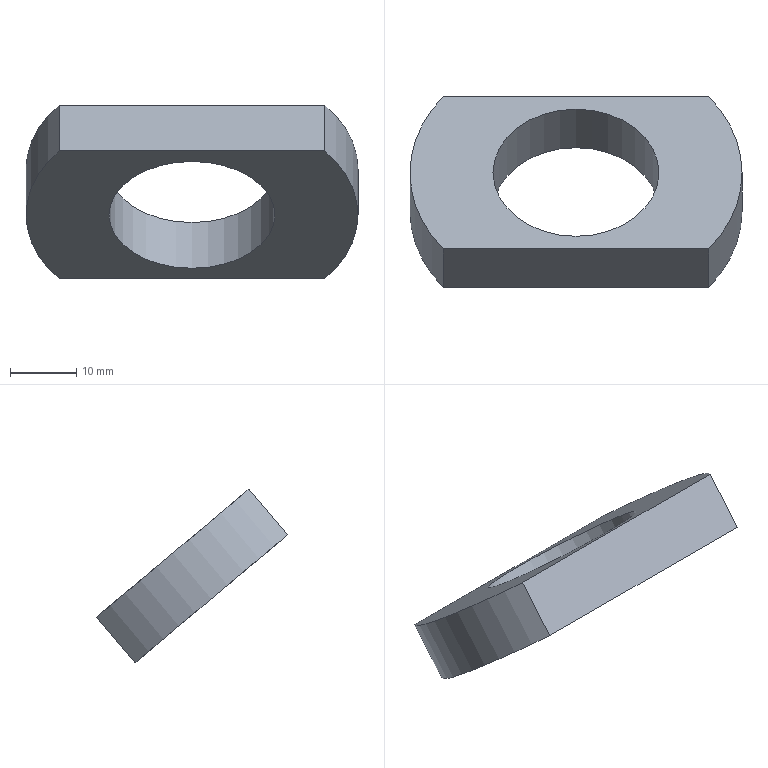Part | NX | features solid 2 | 1 solid | 7 faces | box 50 x 28.766 x 26.178 mm | volume 8222 mm3 | plane 4 | cylinder 3 | commonest cylinder face diameters 50 x2 25 x1
STEP:
#1=CARTESIAN_POINT('',(325.,391.584,-62.275));
#2=VERTEX_POINT('',#1);
#3=CARTESIAN_POINT('',(325.,414.565,-81.558));
#4=VERTEX_POINT('',#3);
#5=CARTESIAN_POINT('',(305.,403.074,-71.917));
#6=DIRECTION('',(0.,0.6428,0.766));
#7=DIRECTION('',(1.,0.,0.));
#8=AXIS2_PLACEMENT_3D('',#5,#6,#7);
#9=CIRCLE('',#8,25.);
#10=EDGE_CURVE('',#2,#4,#9,.T.);
#11=ORIENTED_EDGE('',*,*,#10,.F.);
#12=CARTESIAN_POINT('',(325.,385.799,-69.169));
#13=VERTEX_POINT('',#12);
#14=CARTESIAN_POINT('',(325.,391.584,-62.275));
#15=DIRECTION('',(0.,-0.6428,-0.766));
#16=VECTOR('',#15,1000.);
#17=LINE('',#14,#16);
#18=EDGE_CURVE('',#2,#13,#17,.T.);
#19=ORIENTED_EDGE('',*,*,#18,.T.);
#20=CARTESIAN_POINT('',(325.,408.78,-88.453));
#21=VERTEX_POINT('',#20);
#22=CARTESIAN_POINT('',(305.,397.289,-78.811));
#23=DIRECTION('',(0.,0.6428,0.766));
#24=DIRECTION('',(1.,0.,0.));
#25=AXIS2_PLACEMENT_3D('',#22,#23,#24);
#26=CIRCLE('',#25,25.);
#27=EDGE_CURVE('',#13,#21,#26,.T.);
#28=ORIENTED_EDGE('',*,*,#27,.T.);
#29=CARTESIAN_POINT('',(325.,414.565,-81.558));
#30=DIRECTION('',(0.,-0.6428,-0.766));
#31=VECTOR('',#30,1000.);
#32=LINE('',#29,#31);
#33=EDGE_CURVE('',#4,#21,#32,.T.);
#34=ORIENTED_EDGE('',*,*,#33,.F.);
#35=EDGE_LOOP('',(#11,#19,#28,#34));
#36=FACE_BOUND('',#35,.T.);
#37=CARTESIAN_POINT('',(305.,403.074,-71.917));
#38=DIRECTION('',(0.,-0.6428,-0.766));
#39=DIRECTION('',(-1.,0.,0.));
#40=AXIS2_PLACEMENT_3D('',#37,#38,#39);
#41=CYLINDRICAL_SURFACE('',#40,25.);
#42=ADVANCED_FACE('',(#36),#41,.T.);
#43=CARTESIAN_POINT('',(285.,408.78,-88.453));
#44=VERTEX_POINT('',#43);
#45=CARTESIAN_POINT('',(285.,385.799,-69.169));
#46=VERTEX_POINT('',#45);
#47=CARTESIAN_POINT('',(305.,397.289,-78.811));
#48=DIRECTION('',(0.,0.6428,0.766));
#49=DIRECTION('',(1.,0.,0.));
#50=AXIS2_PLACEMENT_3D('',#47,#48,#49);
#51=CIRCLE('',#50,25.);
#52=EDGE_CURVE('',#44,#46,#51,.T.);
#53=ORIENTED_EDGE('',*,*,#52,.T.);
#54=CARTESIAN_POINT('',(285.,391.584,-62.275));
#55=VERTEX_POINT('',#54);
#56=CARTESIAN_POINT('',(285.,391.584,-62.275));
#57=DIRECTION('',(0.,-0.6428,-0.766));
#58=VECTOR('',#57,1000.);
#59=LINE('',#56,#58);
#60=EDGE_CURVE('',#46,#55,#59,.F.);
#61=ORIENTED_EDGE('',*,*,#60,.T.);
#62=CARTESIAN_POINT('',(285.,414.565,-81.558));
#63=VERTEX_POINT('',#62);
#64=CARTESIAN_POINT('',(305.,403.074,-71.917));
#65=DIRECTION('',(0.,0.6428,0.766));
#66=DIRECTION('',(1.,0.,0.));
#67=AXIS2_PLACEMENT_3D('',#64,#65,#66);
#68=CIRCLE('',#67,25.);
#69=EDGE_CURVE('',#63,#55,#68,.T.);
#70=ORIENTED_EDGE('',*,*,#69,.F.);
#71=CARTESIAN_POINT('',(285.,414.565,-81.558));
#72=DIRECTION('',(0.,-0.6428,-0.766));
#73=VECTOR('',#72,1000.);
#74=LINE('',#71,#73);
#75=EDGE_CURVE('',#44,#63,#74,.F.);
#76=ORIENTED_EDGE('',*,*,#75,.F.);
#77=EDGE_LOOP('',(#53,#61,#70,#76));
#78=FACE_BOUND('',#77,.T.);
#79=CARTESIAN_POINT('',(305.,403.074,-71.917));
#80=DIRECTION('',(0.,-0.6428,-0.766));
#81=DIRECTION('',(-1.,0.,0.));
#82=AXIS2_PLACEMENT_3D('',#79,#80,#81);
#83=CYLINDRICAL_SURFACE('',#82,25.);
#84=ADVANCED_FACE('',(#78),#83,.T.);
#85=CARTESIAN_POINT('',(305.,391.584,-62.275));
#86=DIRECTION('',(-1.,0.,0.));
#87=VECTOR('',#86,1000.);
#88=LINE('',#85,#87);
#89=EDGE_CURVE('',#2,#55,#88,.T.);
#90=ORIENTED_EDGE('',*,*,#89,.F.);
#91=ORIENTED_EDGE('',*,*,#10,.T.);
#92=CARTESIAN_POINT('',(305.,414.565,-81.558));
#93=DIRECTION('',(-1.,0.,0.));
#94=VECTOR('',#93,1000.);
#95=LINE('',#92,#94);
#96=EDGE_CURVE('',#4,#63,#95,.T.);
#97=ORIENTED_EDGE('',*,*,#96,.T.);
#98=ORIENTED_EDGE('',*,*,#69,.T.);
#99=EDGE_LOOP('',(#90,#91,#97,#98));
#100=FACE_BOUND('',#99,.T.);
#101=CARTESIAN_POINT('',(317.5,403.074,-71.917));
#102=VERTEX_POINT('',#101);
#103=CARTESIAN_POINT('',(305.,403.074,-71.917));
#104=DIRECTION('',(0.,0.6428,0.766));
#105=DIRECTION('',(1.,0.,0.));
#106=AXIS2_PLACEMENT_3D('',#103,#104,#105);
#107=CIRCLE('',#106,12.5);
#108=EDGE_CURVE('',#102,#102,#107,.T.);
#109=ORIENTED_EDGE('',*,*,#108,.F.);
#110=EDGE_LOOP('',(#109));
#111=FACE_BOUND('',#110,.T.);
#112=CARTESIAN_POINT('',(305.,403.074,-71.917));
#113=DIRECTION('',(0.,0.6428,0.766));
#114=DIRECTION('',(1.,0.,0.));
#115=AXIS2_PLACEMENT_3D('',#112,#113,#114);
#116=PLANE('',#115);
#117=ADVANCED_FACE('',(#100,#111),#116,.T.);
#118=CARTESIAN_POINT('',(317.5,397.289,-78.811));
#119=VERTEX_POINT('',#118);
#120=CARTESIAN_POINT('',(305.,397.289,-78.811));
#121=DIRECTION('',(0.,0.6428,0.766));
#122=DIRECTION('',(1.,0.,0.));
#123=AXIS2_PLACEMENT_3D('',#120,#121,#122);
#124=CIRCLE('',#123,12.5);
#125=EDGE_CURVE('',#119,#119,#124,.T.);
#126=ORIENTED_EDGE('',*,*,#125,.T.);
#127=EDGE_LOOP('',(#126));
#128=FACE_BOUND('',#127,.T.);
#129=ORIENTED_EDGE('',*,*,#27,.F.);
#130=CARTESIAN_POINT('',(305.,385.799,-69.169));
#131=DIRECTION('',(-1.,0.,0.));
#132=VECTOR('',#131,1000.);
#133=LINE('',#130,#132);
#134=EDGE_CURVE('',#13,#46,#133,.T.);
#135=ORIENTED_EDGE('',*,*,#134,.T.);
#136=ORIENTED_EDGE('',*,*,#52,.F.);
#137=CARTESIAN_POINT('',(305.,408.78,-88.453));
#138=DIRECTION('',(-1.,0.,0.));
#139=VECTOR('',#138,1000.);
#140=LINE('',#137,#139);
#141=EDGE_CURVE('',#21,#44,#140,.T.);
#142=ORIENTED_EDGE('',*,*,#141,.F.);
#143=EDGE_LOOP('',(#129,#135,#136,#142));
#144=FACE_BOUND('',#143,.T.);
#145=CARTESIAN_POINT('',(305.,397.289,-78.811));
#146=DIRECTION('',(0.,0.6428,0.766));
#147=DIRECTION('',(1.,0.,0.));
#148=AXIS2_PLACEMENT_3D('',#145,#146,#147);
#149=PLANE('',#148);
#150=ADVANCED_FACE('',(#128,#144),#149,.F.);
#151=ORIENTED_EDGE('',*,*,#108,.T.);
#152=EDGE_LOOP('',(#151));
#153=FACE_BOUND('',#152,.T.);
#154=ORIENTED_EDGE('',*,*,#125,.F.);
#155=EDGE_LOOP('',(#154));
#156=FACE_BOUND('',#155,.T.);
#157=CARTESIAN_POINT('',(305.,403.074,-71.917));
#158=DIRECTION('',(0.,-0.6428,-0.766));
#159=DIRECTION('',(-1.,0.,0.));
#160=AXIS2_PLACEMENT_3D('',#157,#158,#159);
#161=CYLINDRICAL_SURFACE('',#160,12.5);
#162=ADVANCED_FACE('',(#153,#156),#161,.F.);
#163=ORIENTED_EDGE('',*,*,#96,.F.);
#164=ORIENTED_EDGE('',*,*,#33,.T.);
#165=ORIENTED_EDGE('',*,*,#141,.T.);
#166=ORIENTED_EDGE('',*,*,#75,.T.);
#167=EDGE_LOOP('',(#163,#164,#165,#166));
#168=FACE_BOUND('',#167,.T.);
#169=CARTESIAN_POINT('',(1714.572,408.78,-88.453));
#170=DIRECTION('',(0.,0.766,-0.6428));
#171=DIRECTION('',(0.,0.6428,0.766));
#172=AXIS2_PLACEMENT_3D('',#169,#170,#171);
#173=PLANE('',#172);
#174=ADVANCED_FACE('',(#168),#173,.T.);
#175=ORIENTED_EDGE('',*,*,#89,.T.);
#176=ORIENTED_EDGE('',*,*,#60,.F.);
#177=ORIENTED_EDGE('',*,*,#134,.F.);
#178=ORIENTED_EDGE('',*,*,#18,.F.);
#179=EDGE_LOOP('',(#175,#176,#177,#178));
#180=FACE_BOUND('',#179,.T.);
#181=CARTESIAN_POINT('',(1714.572,385.799,-69.169));
#182=DIRECTION('',(0.,0.766,-0.6428));
#183=DIRECTION('',(0.,0.6428,0.766));
#184=AXIS2_PLACEMENT_3D('',#181,#182,#183);
#185=PLANE('',#184);
#186=ADVANCED_FACE('',(#180),#185,.F.);
#187=CLOSED_SHELL('',(#42,#84,#117,#150,#162,#174,#186));
#188=MANIFOLD_SOLID_BREP('',#187);
#189=(LENGTH_UNIT()NAMED_UNIT(*)SI_UNIT(.MILLI.,.METRE.));
#190=UNCERTAINTY_MEASURE_WITH_UNIT(LENGTH_MEASURE(0.00001),#189,'','');
#191=(NAMED_UNIT(*)PLANE_ANGLE_UNIT()SI_UNIT($,.RADIAN.));
#192=(NAMED_UNIT(*)SI_UNIT($,.STERADIAN.)SOLID_ANGLE_UNIT());
#193=(GEOMETRIC_REPRESENTATION_CONTEXT(3)GLOBAL_UNCERTAINTY_ASSIGNED_CONTEXT((#190))GLOBAL_UNIT_ASSIGNED_CONTEXT((#189,#191,#192))REPRESENTATION_CONTEXT('',''));
#194=ADVANCED_BREP_SHAPE_REPRESENTATION('',(#188),#193);